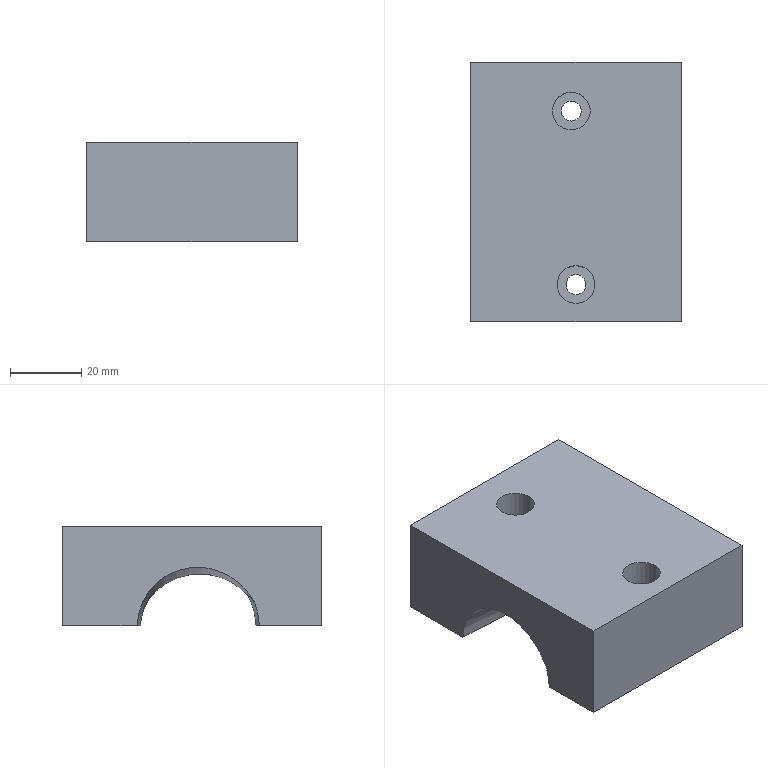NC program | NX | posted with a generic post | part box 59.014 x 72.744 x 27.972 mm
Lines 94104 to 94199 of 94199:
(ZLEVEL_PROFILE_1_COPY , TOOL : D6A45)
N188182 T01 M6
N188184 G54
N188186 G17 G0 G90 X-23.309 Y1.524 S9500 M3
N188188 G43 Z30. H1
N188190 Z0.5
N188192 G94 G1 Z-1. F1250.
N188194 X-24.242 Y1.839
N188196 G3 X-24.542 Y1.319 R0.6
N188198 X-22.701 Y-0.522 R1.841
N188200 X-24.542 Y1.319 R-1.841
N188202 X-24.242 Y0.8 R0.6
N188204 G1 X-23.309 Y1.115
N188206 Z0.5
N188208 G0 Z30.
N188210 X-22.631 Y19.577
N188212 Z0.5
N188214 G1 Z-1.
N188216 X-22.352 Y20.513
N188218 G3 X-22.872 Y20.813 R0.6
N188220 X-24.913 Y18.771 R2.041
N188222 X-22.872 Y20.813 R-2.041
N188224 X-23.391 Y20.513 R0.6
N188226 G1 X-23.112 Y19.577
N188228 Z0.5
N188230 G0 Z30.
N188232 X26.588 Y-0.205
N188234 Z0.5
N188236 G1 Z-1.
N188238 X27.522 Y-0.52
N188240 G3 X27.822 Y0. R0.6
N188242 X25.98 Y1.841 R1.841
N188244 X27.822 Y0. R-1.841
N188246 X27.522 Y0.52 R0.6
N188248 G1 X26.588 Y0.205
N188250 Z0.5
N188252 G0 Z30.
N188254 X26.786 Y-17.248
N188256 Z0.5
N188258 G1 Z-1.
N188260 X27.722 Y-17.527
N188262 G3 X28.022 Y-17.007 R0.6
N188264 X25.98 Y-14.966 R2.041
N188266 X28.022 Y-17.007 R-2.041
N188268 X27.722 Y-16.487 R0.6
N188270 G1 X26.786 Y-16.766
N188272 Z0.5
N188274 G0 Z30.
N188276 X38.53 Y1.035
N188278 Z0.5
N188280 G1 Z-1.
N188282 X37.63 Y0.516
N188284 G3 X37.33 Y-0.004 R0.6
N188286 G1 Y-29.518
N188288 G2 X36.374 Y-30.466 R0.952
N188290 G1 X19.421
N188292 G2 X18.493 Y-29.346 R0.945
N188294 G3 X19.517 Y-18.537 R59.389
N188296 G2 X17.657 Y4.97 R81.145
N188298 G3 X17.566 Y7.845 R15.112
N188300 G2 X17.911 Y29.66 R79.956
N188302 X18.854 Y30.466 R0.972
N188304 G1 X36.374
N188306 G2 X37.33 Y29.51 R0.979
N188308 G1 Y-0.004
N188310 G3 X37.63 Y-0.524 R0.6
N188312 G1 X38.53 Y-1.043
N188314 Z0.5
N188316 G0 Z30.
N188318 X-38.53
N188320 Z0.5
N188322 G1 Z-1.
N188324 X-37.63 Y-0.524
N188326 G3 X-37.33 Y-0.004 R0.6
N188328 G1 Y29.51
N188330 G2 X-36.374 Y30.466 R0.979
N188332 G1 X-15.376
N188334 G2 X-14.436 Y29.573 R0.941
N188336 G1 X-14.354 Y27.969
N188338 X-13.78 Y17.822
N188340 X-13.656 Y15.286
N188342 G2 X-14.289 Y-5.008 R122.226
N188344 G3 X-15.323 Y-16.845 R216.
N188346 X-14.626 Y-29.373 R53.725
N188348 G2 X-15.544 Y-30.466 R0.932
N188350 G1 X-36.374
N188352 G2 X-37.33 Y-29.518 R0.952
N188354 G1 Y-0.004
N188356 G3 X-37.63 Y0.516 R0.6
N188358 G1 X-38.53 Y1.035
N188360 Z0.5
N188362 G0 Z30.
N188364 M5
N188366 M2